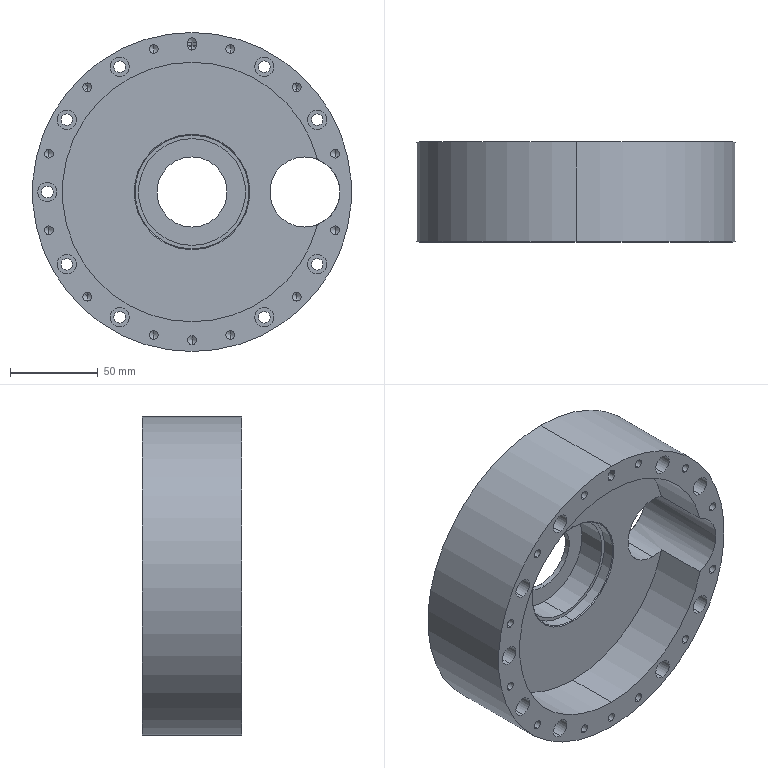Part | SolidWorks | features HoleWzd 7, Chamfer 2, ICE 2, Cut 1, MoveFace 1, Revolution 1 | 1 solid | 143 faces | box 182 x 57 x 182 mm | volume 783289 mm3 | cylinder 83 | cone 38 | plane 22 | commonest cylinder face diameters 5 x29 6.6 x18 11 x18 6 x5 40 x4 148 x3